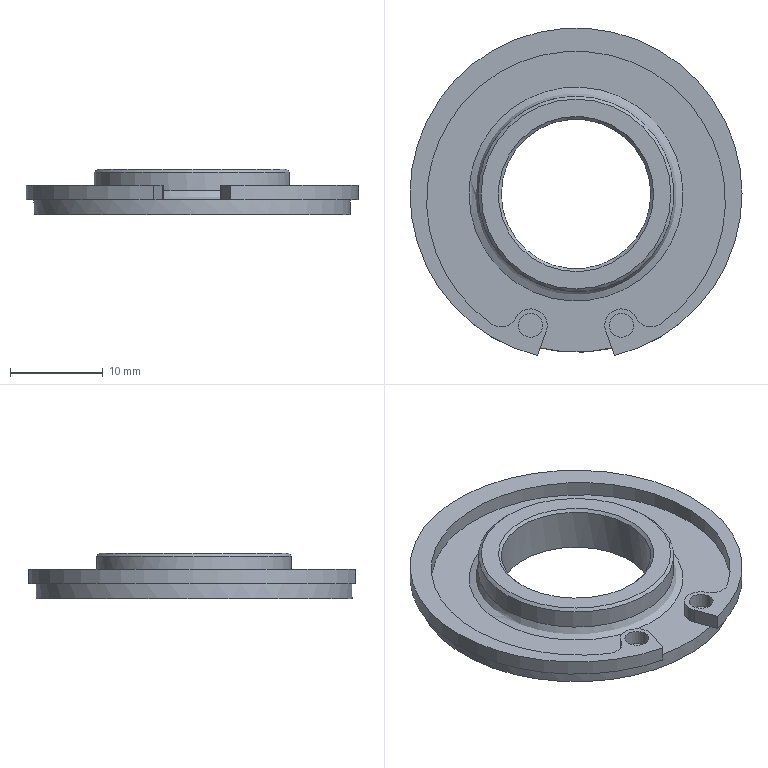Part | NX | features CDQ2B32-35DM_CQ2 SnapRing_32 2 | 1 solid | 23 faces | box 35.7 x 35.209 x 4.9 mm | volume 1920 mm3 | cylinder 11 | plane 9 | cone 2 | spline 1 | commonest cylinder face diameters 3.57 x4 2.57 x2 16.1 x1 21 x1 32.13 x1 34 x1